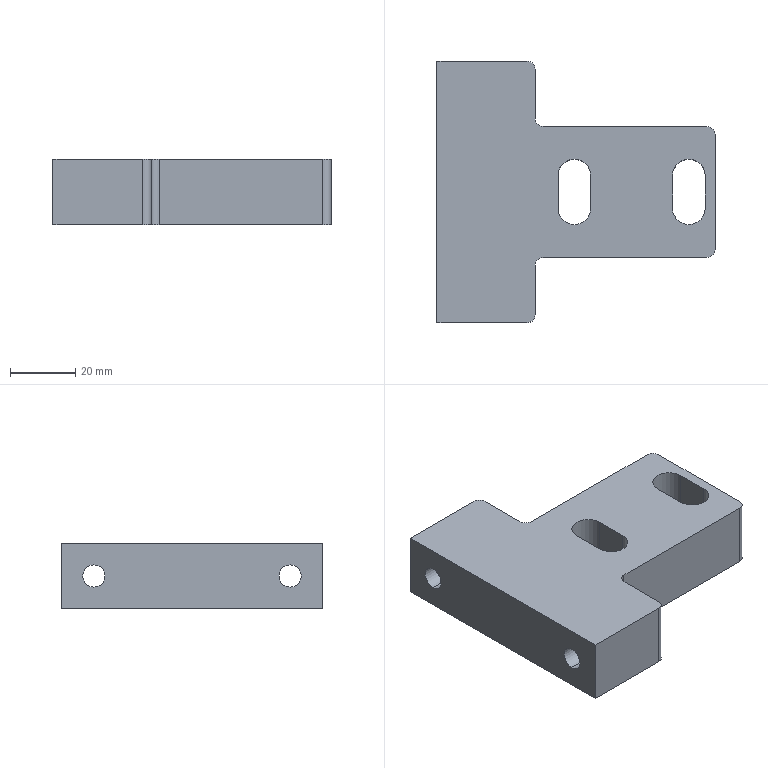Part | 1 solid | 28 faces | box 85 x 80 x 20 mm | volume 82626 mm3 | cylinder 14 | plane 14 | commonest cylinder face diameters 5 x6 6.8 x4 10 x4
STEP:
#1=CARTESIAN_POINT('',(-42.5,30.,13.4));
#2=VERTEX_POINT('',#1);
#3=CARTESIAN_POINT('',(-42.5,30.,6.6));
#4=VERTEX_POINT('',#3);
#5=CARTESIAN_POINT('',(-42.5,30.,10.));
#6=DIRECTION('',(1.,0.,0.));
#7=DIRECTION('',(0.,0.,-1.));
#8=AXIS2_PLACEMENT_3D('',#5,#6,#7);
#9=CIRCLE('',#8,3.4);
#10=EDGE_CURVE('',#2,#4,#9,.T.);
#11=ORIENTED_EDGE('',*,*,#10,.F.);
#12=CARTESIAN_POINT('',(-12.5,30.,13.4));
#13=VERTEX_POINT('',#12);
#14=CARTESIAN_POINT('',(-12.5,30.,13.4));
#15=DIRECTION('',(1.,0.,0.));
#16=VECTOR('',#15,1000.);
#17=LINE('',#14,#16);
#18=EDGE_CURVE('',#2,#13,#17,.T.);
#19=ORIENTED_EDGE('',*,*,#18,.T.);
#20=CARTESIAN_POINT('',(-12.5,30.,6.6));
#21=VERTEX_POINT('',#20);
#22=CARTESIAN_POINT('',(-12.5,30.,10.));
#23=DIRECTION('',(1.,0.,0.));
#24=DIRECTION('',(0.,0.,-1.));
#25=AXIS2_PLACEMENT_3D('',#22,#23,#24);
#26=CIRCLE('',#25,3.4);
#27=EDGE_CURVE('',#13,#21,#26,.T.);
#28=ORIENTED_EDGE('',*,*,#27,.T.);
#29=CARTESIAN_POINT('',(-12.5,30.,6.6));
#30=DIRECTION('',(1.,0.,0.));
#31=VECTOR('',#30,1000.);
#32=LINE('',#29,#31);
#33=EDGE_CURVE('',#4,#21,#32,.T.);
#34=ORIENTED_EDGE('',*,*,#33,.F.);
#35=EDGE_LOOP('',(#11,#19,#28,#34));
#36=FACE_OUTER_BOUND('',#35,.T.);
#37=CARTESIAN_POINT('',(-12.5,30.,10.));
#38=DIRECTION('',(1.,0.,0.));
#39=DIRECTION('',(0.,0.,-1.));
#40=AXIS2_PLACEMENT_3D('',#37,#38,#39);
#41=CYLINDRICAL_SURFACE('',#40,3.4);
#42=ADVANCED_FACE('',(#36),#41,.F.);
#43=CARTESIAN_POINT('',(-42.5,-30.,13.4));
#44=VERTEX_POINT('',#43);
#45=CARTESIAN_POINT('',(-42.5,-30.,6.6));
#46=VERTEX_POINT('',#45);
#47=CARTESIAN_POINT('',(-42.5,-30.,10.));
#48=DIRECTION('',(1.,0.,0.));
#49=DIRECTION('',(0.,0.,-1.));
#50=AXIS2_PLACEMENT_3D('',#47,#48,#49);
#51=CIRCLE('',#50,3.4);
#52=EDGE_CURVE('',#44,#46,#51,.T.);
#53=ORIENTED_EDGE('',*,*,#52,.F.);
#54=CARTESIAN_POINT('',(-12.5,-30.,13.4));
#55=VERTEX_POINT('',#54);
#56=CARTESIAN_POINT('',(-12.5,-30.,13.4));
#57=DIRECTION('',(1.,0.,0.));
#58=VECTOR('',#57,1000.);
#59=LINE('',#56,#58);
#60=EDGE_CURVE('',#44,#55,#59,.T.);
#61=ORIENTED_EDGE('',*,*,#60,.T.);
#62=CARTESIAN_POINT('',(-12.5,-30.,6.6));
#63=VERTEX_POINT('',#62);
#64=CARTESIAN_POINT('',(-12.5,-30.,10.));
#65=DIRECTION('',(1.,0.,0.));
#66=DIRECTION('',(0.,0.,-1.));
#67=AXIS2_PLACEMENT_3D('',#64,#65,#66);
#68=CIRCLE('',#67,3.4);
#69=EDGE_CURVE('',#55,#63,#68,.T.);
#70=ORIENTED_EDGE('',*,*,#69,.T.);
#71=CARTESIAN_POINT('',(-12.5,-30.,6.6));
#72=DIRECTION('',(1.,0.,0.));
#73=VECTOR('',#72,1000.);
#74=LINE('',#71,#73);
#75=EDGE_CURVE('',#46,#63,#74,.T.);
#76=ORIENTED_EDGE('',*,*,#75,.F.);
#77=EDGE_LOOP('',(#53,#61,#70,#76));
#78=FACE_OUTER_BOUND('',#77,.T.);
#79=CARTESIAN_POINT('',(-12.5,-30.,10.));
#80=DIRECTION('',(1.,0.,0.));
#81=DIRECTION('',(0.,0.,-1.));
#82=AXIS2_PLACEMENT_3D('',#79,#80,#81);
#83=CYLINDRICAL_SURFACE('',#82,3.4);
#84=ADVANCED_FACE('',(#78),#83,.F.);
#85=CARTESIAN_POINT('',(-12.5,-22.5,20.));
#86=VERTEX_POINT('',#85);
#87=CARTESIAN_POINT('',(-12.5,-37.5,20.));
#88=VERTEX_POINT('',#87);
#89=CARTESIAN_POINT('',(-12.5,-40.,20.));
#90=DIRECTION('',(0.,-1.,0.));
#91=VECTOR('',#90,1000.);
#92=LINE('',#89,#91);
#93=EDGE_CURVE('',#86,#88,#92,.T.);
#94=ORIENTED_EDGE('',*,*,#93,.T.);
#95=CARTESIAN_POINT('',(-12.5,-37.5,0.));
#96=VERTEX_POINT('',#95);
#97=CARTESIAN_POINT('',(-12.5,-37.5,0.));
#98=DIRECTION('',(0.,0.,-1.));
#99=VECTOR('',#98,1000.);
#100=LINE('',#97,#99);
#101=EDGE_CURVE('',#88,#96,#100,.T.);
#102=ORIENTED_EDGE('',*,*,#101,.T.);
#103=CARTESIAN_POINT('',(-12.5,-22.5,0.));
#104=VERTEX_POINT('',#103);
#105=CARTESIAN_POINT('',(-12.5,-40.,0.));
#106=DIRECTION('',(0.,-1.,0.));
#107=VECTOR('',#106,1000.);
#108=LINE('',#105,#107);
#109=EDGE_CURVE('',#104,#96,#108,.T.);
#110=ORIENTED_EDGE('',*,*,#109,.F.);
#111=CARTESIAN_POINT('',(-12.5,-22.5,20.));
#112=DIRECTION('',(0.,0.,1.));
#113=VECTOR('',#112,1000.);
#114=LINE('',#111,#113);
#115=EDGE_CURVE('',#104,#86,#114,.T.);
#116=ORIENTED_EDGE('',*,*,#115,.T.);
#117=EDGE_LOOP('',(#94,#102,#110,#116));
#118=FACE_OUTER_BOUND('',#117,.T.);
#119=CARTESIAN_POINT('',(-12.5,-30.,10.));
#120=DIRECTION('',(1.,0.,0.));
#121=DIRECTION('',(0.,0.,-1.));
#122=AXIS2_PLACEMENT_3D('',#119,#120,#121);
#123=CIRCLE('',#122,3.4);
#124=EDGE_CURVE('',#63,#55,#123,.T.);
#125=ORIENTED_EDGE('',*,*,#124,.F.);
#126=ORIENTED_EDGE('',*,*,#69,.F.);
#127=EDGE_LOOP('',(#125,#126));
#128=FACE_BOUND('',#127,.T.);
#129=CARTESIAN_POINT('',(-12.5,-40.,0.));
#130=DIRECTION('',(-1.,0.,0.));
#131=DIRECTION('',(0.,0.,1.));
#132=AXIS2_PLACEMENT_3D('',#129,#130,#131);
#133=PLANE('',#132);
#134=ADVANCED_FACE('',(#118,#128),#133,.F.);
#135=CARTESIAN_POINT('',(42.5,-17.5,20.));
#136=VERTEX_POINT('',#135);
#137=CARTESIAN_POINT('',(42.5,17.5,20.));
#138=VERTEX_POINT('',#137);
#139=CARTESIAN_POINT('',(42.5,-40.,20.));
#140=DIRECTION('',(0.,1.,0.));
#141=VECTOR('',#140,1000.);
#142=LINE('',#139,#141);
#143=EDGE_CURVE('',#136,#138,#142,.T.);
#144=ORIENTED_EDGE('',*,*,#143,.F.);
#145=CARTESIAN_POINT('',(42.5,-17.5,0.));
#146=VERTEX_POINT('',#145);
#147=CARTESIAN_POINT('',(42.5,-17.5,20.));
#148=DIRECTION('',(0.,0.,-1.));
#149=VECTOR('',#148,1000.);
#150=LINE('',#147,#149);
#151=EDGE_CURVE('',#136,#146,#150,.T.);
#152=ORIENTED_EDGE('',*,*,#151,.T.);
#153=CARTESIAN_POINT('',(42.5,17.5,0.));
#154=VERTEX_POINT('',#153);
#155=CARTESIAN_POINT('',(42.5,-40.,0.));
#156=DIRECTION('',(0.,1.,0.));
#157=VECTOR('',#156,1000.);
#158=LINE('',#155,#157);
#159=EDGE_CURVE('',#146,#154,#158,.T.);
#160=ORIENTED_EDGE('',*,*,#159,.T.);
#161=CARTESIAN_POINT('',(42.5,17.5,20.));
#162=DIRECTION('',(0.,0.,1.));
#163=VECTOR('',#162,1000.);
#164=LINE('',#161,#163);
#165=EDGE_CURVE('',#154,#138,#164,.T.);
#166=ORIENTED_EDGE('',*,*,#165,.T.);
#167=EDGE_LOOP('',(#144,#152,#160,#166));
#168=FACE_OUTER_BOUND('',#167,.T.);
#169=CARTESIAN_POINT('',(42.5,-40.,20.));
#170=DIRECTION('',(-1.,0.,0.));
#171=DIRECTION('',(0.,0.,1.));
#172=AXIS2_PLACEMENT_3D('',#169,#170,#171);
#173=PLANE('',#172);
#174=ADVANCED_FACE('',(#168),#173,.F.);
#175=CARTESIAN_POINT('',(-15.,40.,20.));
#176=VERTEX_POINT('',#175);
#177=CARTESIAN_POINT('',(-42.5,40.,20.));
#178=VERTEX_POINT('',#177);
#179=CARTESIAN_POINT('',(-42.5,40.,20.));
#180=DIRECTION('',(-1.,0.,0.));
#181=VECTOR('',#180,1000.);
#182=LINE('',#179,#181);
#183=EDGE_CURVE('',#176,#178,#182,.T.);
#184=ORIENTED_EDGE('',*,*,#183,.F.);
#185=CARTESIAN_POINT('',(-15.,40.,0.));
#186=VERTEX_POINT('',#185);
#187=CARTESIAN_POINT('',(-15.,40.,20.));
#188=DIRECTION('',(0.,0.,-1.));
#189=VECTOR('',#188,1000.);
#190=LINE('',#187,#189);
#191=EDGE_CURVE('',#176,#186,#190,.T.);
#192=ORIENTED_EDGE('',*,*,#191,.T.);
#193=CARTESIAN_POINT('',(-42.5,40.,0.));
#194=VERTEX_POINT('',#193);
#195=CARTESIAN_POINT('',(-42.5,40.,0.));
#196=DIRECTION('',(-1.,0.,0.));
#197=VECTOR('',#196,1000.);
#198=LINE('',#195,#197);
#199=EDGE_CURVE('',#186,#194,#198,.T.);
#200=ORIENTED_EDGE('',*,*,#199,.T.);
#201=CARTESIAN_POINT('',(-42.5,40.,20.));
#202=DIRECTION('',(0.,0.,-1.));
#203=VECTOR('',#202,1000.);
#204=LINE('',#201,#203);
#205=EDGE_CURVE('',#178,#194,#204,.T.);
#206=ORIENTED_EDGE('',*,*,#205,.F.);
#207=EDGE_LOOP('',(#184,#192,#200,#206));
#208=FACE_OUTER_BOUND('',#207,.T.);
#209=CARTESIAN_POINT('',(-42.5,40.,20.));
#210=DIRECTION('',(0.,-1.,0.));
#211=DIRECTION('',(0.,0.,-1.));
#212=AXIS2_PLACEMENT_3D('',#209,#210,#211);
#213=PLANE('',#212);
#214=ADVANCED_FACE('',(#208),#213,.F.);
#215=CARTESIAN_POINT('',(-42.5,30.,10.));
#216=DIRECTION('',(1.,0.,0.));
#217=DIRECTION('',(0.,0.,-1.));
#218=AXIS2_PLACEMENT_3D('',#215,#216,#217);
#219=CIRCLE('',#218,3.4);
#220=EDGE_CURVE('',#4,#2,#219,.T.);
#221=ORIENTED_EDGE('',*,*,#220,.T.);
#222=ORIENTED_EDGE('',*,*,#10,.T.);
#223=EDGE_LOOP('',(#221,#222));
#224=FACE_BOUND('',#223,.T.);
#225=CARTESIAN_POINT('',(-42.5,-30.,10.));
#226=DIRECTION('',(1.,0.,0.));
#227=DIRECTION('',(0.,0.,-1.));
#228=AXIS2_PLACEMENT_3D('',#225,#226,#227);
#229=CIRCLE('',#228,3.4);
#230=EDGE_CURVE('',#46,#44,#229,.T.);
#231=ORIENTED_EDGE('',*,*,#230,.T.);
#232=ORIENTED_EDGE('',*,*,#52,.T.);
#233=EDGE_LOOP('',(#231,#232));
#234=FACE_BOUND('',#233,.T.);
#235=CARTESIAN_POINT('',(-42.5,-40.,0.));
#236=VERTEX_POINT('',#235);
#237=CARTESIAN_POINT('',(-42.5,-40.,0.));
#238=DIRECTION('',(0.,-1.,0.));
#239=VECTOR('',#238,1000.);
#240=LINE('',#237,#239);
#241=EDGE_CURVE('',#194,#236,#240,.T.);
#242=ORIENTED_EDGE('',*,*,#241,.T.);
#243=CARTESIAN_POINT('',(-42.5,-40.,20.));
#244=VERTEX_POINT('',#243);
#245=CARTESIAN_POINT('',(-42.5,-40.,20.));
#246=DIRECTION('',(0.,0.,-1.));
#247=VECTOR('',#246,1000.);
#248=LINE('',#245,#247);
#249=EDGE_CURVE('',#244,#236,#248,.T.);
#250=ORIENTED_EDGE('',*,*,#249,.F.);
#251=CARTESIAN_POINT('',(-42.5,-40.,20.));
#252=DIRECTION('',(0.,-1.,0.));
#253=VECTOR('',#252,1000.);
#254=LINE('',#251,#253);
#255=EDGE_CURVE('',#178,#244,#254,.T.);
#256=ORIENTED_EDGE('',*,*,#255,.F.);
#257=ORIENTED_EDGE('',*,*,#205,.T.);
#258=EDGE_LOOP('',(#242,#250,#256,#257));
#259=FACE_OUTER_BOUND('',#258,.T.);
#260=CARTESIAN_POINT('',(-42.5,-40.,20.));
#261=DIRECTION('',(1.,0.,0.));
#262=DIRECTION('',(0.,0.,-1.));
#263=AXIS2_PLACEMENT_3D('',#260,#261,#262);
#264=PLANE('',#263);
#265=ADVANCED_FACE('',(#224,#234,#259),#264,.F.);
#266=CARTESIAN_POINT('',(-15.,-40.,0.));
#267=VERTEX_POINT('',#266);
#268=CARTESIAN_POINT('',(-42.5,-40.,0.));
#269=DIRECTION('',(1.,0.,0.));
#270=VECTOR('',#269,1000.);
#271=LINE('',#268,#270);
#272=EDGE_CURVE('',#236,#267,#271,.T.);
#273=ORIENTED_EDGE('',*,*,#272,.T.);
#274=CARTESIAN_POINT('',(-15.,-40.,20.));
#275=VERTEX_POINT('',#274);
#276=CARTESIAN_POINT('',(-15.,-40.,20.));
#277=DIRECTION('',(0.,0.,1.));
#278=VECTOR('',#277,1000.);
#279=LINE('',#276,#278);
#280=EDGE_CURVE('',#267,#275,#279,.T.);
#281=ORIENTED_EDGE('',*,*,#280,.T.);
#282=CARTESIAN_POINT('',(-42.5,-40.,20.));
#283=DIRECTION('',(1.,0.,0.));
#284=VECTOR('',#283,1000.);
#285=LINE('',#282,#284);
#286=EDGE_CURVE('',#244,#275,#285,.T.);
#287=ORIENTED_EDGE('',*,*,#286,.F.);
#288=ORIENTED_EDGE('',*,*,#249,.T.);
#289=EDGE_LOOP('',(#273,#281,#287,#288));
#290=FACE_OUTER_BOUND('',#289,.T.);
#291=CARTESIAN_POINT('',(-42.5,-40.,20.));
#292=DIRECTION('',(0.,1.,0.));
#293=DIRECTION('',(0.,0.,1.));
#294=AXIS2_PLACEMENT_3D('',#291,#292,#293);
#295=PLANE('',#294);
#296=ADVANCED_FACE('',(#290),#295,.F.);
#297=CARTESIAN_POINT('',(4.5,-5.,20.));
#298=VERTEX_POINT('',#297);
#299=CARTESIAN_POINT('',(4.5,5.,20.));
#300=VERTEX_POINT('',#299);
#301=CARTESIAN_POINT('',(4.5,-5.,20.));
#302=DIRECTION('',(0.,1.,0.));
#303=VECTOR('',#302,1000.);
#304=LINE('',#301,#303);
#305=EDGE_CURVE('',#298,#300,#304,.T.);
#306=ORIENTED_EDGE('',*,*,#305,.F.);
#307=CARTESIAN_POINT('',(-5.5,-5.,20.));
#308=VERTEX_POINT('',#307);
#309=CARTESIAN_POINT('',(-0.5,-5.,20.));
#310=DIRECTION('',(0.,0.,1.));
#311=DIRECTION('',(1.,0.,0.));
#312=AXIS2_PLACEMENT_3D('',#309,#310,#311);
#313=CIRCLE('',#312,5.);
#314=EDGE_CURVE('',#308,#298,#313,.T.);
#315=ORIENTED_EDGE('',*,*,#314,.F.);
#316=CARTESIAN_POINT('',(-5.5,5.,20.));
#317=VERTEX_POINT('',#316);
#318=CARTESIAN_POINT('',(-5.5,-5.,20.));
#319=DIRECTION('',(0.,-1.,0.));
#320=VECTOR('',#319,1000.);
#321=LINE('',#318,#320);
#322=EDGE_CURVE('',#317,#308,#321,.T.);
#323=ORIENTED_EDGE('',*,*,#322,.F.);
#324=CARTESIAN_POINT('',(-0.5,5.,20.));
#325=DIRECTION('',(0.,0.,1.));
#326=DIRECTION('',(1.,0.,0.));
#327=AXIS2_PLACEMENT_3D('',#324,#325,#326);
#328=CIRCLE('',#327,5.);
#329=EDGE_CURVE('',#300,#317,#328,.T.);
#330=ORIENTED_EDGE('',*,*,#329,.F.);
#331=EDGE_LOOP('',(#306,#315,#323,#330));
#332=FACE_BOUND('',#331,.T.);
#333=CARTESIAN_POINT('',(39.5,-5.,20.));
#334=VERTEX_POINT('',#333);
#335=CARTESIAN_POINT('',(39.5,5.,20.));
#336=VERTEX_POINT('',#335);
#337=CARTESIAN_POINT('',(39.5,-5.,20.));
#338=DIRECTION('',(0.,1.,0.));
#339=VECTOR('',#338,1000.);
#340=LINE('',#337,#339);
#341=EDGE_CURVE('',#334,#336,#340,.T.);
#342=ORIENTED_EDGE('',*,*,#341,.F.);
#343=CARTESIAN_POINT('',(29.5,-5.,20.));
#344=VERTEX_POINT('',#343);
#345=CARTESIAN_POINT('',(34.5,-5.,20.));
#346=DIRECTION('',(0.,0.,1.));
#347=DIRECTION('',(1.,0.,0.));
#348=AXIS2_PLACEMENT_3D('',#345,#346,#347);
#349=CIRCLE('',#348,5.);
#350=EDGE_CURVE('',#344,#334,#349,.T.);
#351=ORIENTED_EDGE('',*,*,#350,.F.);
#352=CARTESIAN_POINT('',(29.5,5.,20.));
#353=VERTEX_POINT('',#352);
#354=CARTESIAN_POINT('',(29.5,-5.,20.));
#355=DIRECTION('',(0.,-1.,0.));
#356=VECTOR('',#355,1000.);
#357=LINE('',#354,#356);
#358=EDGE_CURVE('',#353,#344,#357,.T.);
#359=ORIENTED_EDGE('',*,*,#358,.F.);
#360=CARTESIAN_POINT('',(34.5,5.,20.));
#361=DIRECTION('',(0.,0.,1.));
#362=DIRECTION('',(1.,0.,0.));
#363=AXIS2_PLACEMENT_3D('',#360,#361,#362);
#364=CIRCLE('',#363,5.);
#365=EDGE_CURVE('',#336,#353,#364,.T.);
#366=ORIENTED_EDGE('',*,*,#365,.F.);
#367=EDGE_LOOP('',(#342,#351,#359,#366));
#368=FACE_BOUND('',#367,.T.);
#369=CARTESIAN_POINT('',(-12.5,37.5,20.));
#370=VERTEX_POINT('',#369);
#371=CARTESIAN_POINT('',(-12.5,22.5,20.));
#372=VERTEX_POINT('',#371);
#373=CARTESIAN_POINT('',(-12.5,40.,20.));
#374=DIRECTION('',(0.,-1.,0.));
#375=VECTOR('',#374,1000.);
#376=LINE('',#373,#375);
#377=EDGE_CURVE('',#370,#372,#376,.T.);
#378=ORIENTED_EDGE('',*,*,#377,.F.);
#379=CARTESIAN_POINT('',(-15.,37.5,20.));
#380=DIRECTION('',(0.,0.,1.));
#381=DIRECTION('',(-1.,0.,0.));
#382=AXIS2_PLACEMENT_3D('',#379,#380,#381);
#383=CIRCLE('',#382,2.5);
#384=EDGE_CURVE('',#370,#176,#383,.T.);
#385=ORIENTED_EDGE('',*,*,#384,.T.);
#386=ORIENTED_EDGE('',*,*,#183,.T.);
#387=ORIENTED_EDGE('',*,*,#255,.T.);
#388=ORIENTED_EDGE('',*,*,#286,.T.);
#389=CARTESIAN_POINT('',(-15.,-37.5,20.));
#390=DIRECTION('',(0.,0.,1.));
#391=DIRECTION('',(-1.,0.,0.));
#392=AXIS2_PLACEMENT_3D('',#389,#390,#391);
#393=CIRCLE('',#392,2.5);
#394=EDGE_CURVE('',#275,#88,#393,.T.);
#395=ORIENTED_EDGE('',*,*,#394,.T.);
#396=ORIENTED_EDGE('',*,*,#93,.F.);
#397=CARTESIAN_POINT('',(-10.,-20.,20.));
#398=VERTEX_POINT('',#397);
#399=CARTESIAN_POINT('',(-10.,-22.5,20.));
#400=DIRECTION('',(0.,0.,-1.));
#401=DIRECTION('',(-1.,0.,0.));
#402=AXIS2_PLACEMENT_3D('',#399,#400,#401);
#403=CIRCLE('',#402,2.5);
#404=EDGE_CURVE('',#86,#398,#403,.T.);
#405=ORIENTED_EDGE('',*,*,#404,.T.);
#406=CARTESIAN_POINT('',(40.,-20.,20.));
#407=VERTEX_POINT('',#406);
#408=CARTESIAN_POINT('',(42.5,-20.,20.));
#409=DIRECTION('',(-1.,0.,0.));
#410=VECTOR('',#409,1000.);
#411=LINE('',#408,#410);
#412=EDGE_CURVE('',#407,#398,#411,.T.);
#413=ORIENTED_EDGE('',*,*,#412,.F.);
#414=CARTESIAN_POINT('',(40.,-17.5,20.));
#415=DIRECTION('',(0.,0.,1.));
#416=DIRECTION('',(-1.,0.,0.));
#417=AXIS2_PLACEMENT_3D('',#414,#415,#416);
#418=CIRCLE('',#417,2.5);
#419=EDGE_CURVE('',#407,#136,#418,.T.);
#420=ORIENTED_EDGE('',*,*,#419,.T.);
#421=ORIENTED_EDGE('',*,*,#143,.T.);
#422=CARTESIAN_POINT('',(40.,20.,20.));
#423=VERTEX_POINT('',#422);
#424=CARTESIAN_POINT('',(40.,17.5,20.));
#425=DIRECTION('',(0.,0.,1.));
#426=DIRECTION('',(-1.,0.,0.));
#427=AXIS2_PLACEMENT_3D('',#424,#425,#426);
#428=CIRCLE('',#427,2.5);
#429=EDGE_CURVE('',#138,#423,#428,.T.);
#430=ORIENTED_EDGE('',*,*,#429,.T.);
#431=CARTESIAN_POINT('',(-10.,20.,20.));
#432=VERTEX_POINT('',#431);
#433=CARTESIAN_POINT('',(42.5,20.,20.));
#434=DIRECTION('',(1.,0.,0.));
#435=VECTOR('',#434,1000.);
#436=LINE('',#433,#435);
#437=EDGE_CURVE('',#432,#423,#436,.T.);
#438=ORIENTED_EDGE('',*,*,#437,.F.);
#439=CARTESIAN_POINT('',(-10.,22.5,20.));
#440=DIRECTION('',(0.,0.,-1.));
#441=DIRECTION('',(-1.,0.,0.));
#442=AXIS2_PLACEMENT_3D('',#439,#440,#441);
#443=CIRCLE('',#442,2.5);
#444=EDGE_CURVE('',#432,#372,#443,.T.);
#445=ORIENTED_EDGE('',*,*,#444,.T.);
#446=EDGE_LOOP('',(#378,#385,#386,#387,#388,#395,#396,#405,#413,#420,#421,#430,#438,#445));
#447=FACE_OUTER_BOUND('',#446,.T.);
#448=CARTESIAN_POINT('',(0.,0.,20.));
#449=DIRECTION('',(0.,0.,-1.));
#450=DIRECTION('',(-1.,0.,0.));
#451=AXIS2_PLACEMENT_3D('',#448,#449,#450);
#452=PLANE('',#451);
#453=ADVANCED_FACE('',(#332,#368,#447),#452,.F.);
#454=CARTESIAN_POINT('',(-5.5,-5.,0.));
#455=VERTEX_POINT('',#454);
#456=CARTESIAN_POINT('',(4.5,-5.,0.));
#457=VERTEX_POINT('',#456);
#458=CARTESIAN_POINT('',(-0.5,-5.,0.));
#459=DIRECTION('',(0.,0.,1.));
#460=DIRECTION('',(1.,0.,0.));
#461=AXIS2_PLACEMENT_3D('',#458,#459,#460);
#462=CIRCLE('',#461,5.);
#463=EDGE_CURVE('',#455,#457,#462,.T.);
#464=ORIENTED_EDGE('',*,*,#463,.T.);
#465=CARTESIAN_POINT('',(4.5,5.,0.));
#466=VERTEX_POINT('',#465);
#467=CARTESIAN_POINT('',(4.5,-5.,0.));
#468=DIRECTION('',(0.,1.,0.));
#469=VECTOR('',#468,1000.);
#470=LINE('',#467,#469);
#471=EDGE_CURVE('',#457,#466,#470,.T.);
#472=ORIENTED_EDGE('',*,*,#471,.T.);
#473=CARTESIAN_POINT('',(-5.5,5.,0.));
#474=VERTEX_POINT('',#473);
#475=CARTESIAN_POINT('',(-0.5,5.,0.));
#476=DIRECTION('',(0.,0.,1.));
#477=DIRECTION('',(1.,0.,0.));
#478=AXIS2_PLACEMENT_3D('',#475,#476,#477);
#479=CIRCLE('',#478,5.);
#480=EDGE_CURVE('',#466,#474,#479,.T.);
#481=ORIENTED_EDGE('',*,*,#480,.T.);
#482=CARTESIAN_POINT('',(-5.5,-5.,0.));
#483=DIRECTION('',(0.,-1.,0.));
#484=VECTOR('',#483,1000.);
#485=LINE('',#482,#484);
#486=EDGE_CURVE('',#474,#455,#485,.T.);
#487=ORIENTED_EDGE('',*,*,#486,.T.);
#488=EDGE_LOOP('',(#464,#472,#481,#487));
#489=FACE_BOUND('',#488,.T.);
#490=CARTESIAN_POINT('',(29.5,-5.,0.));
#491=VERTEX_POINT('',#490);
#492=CARTESIAN_POINT('',(39.5,-5.,0.));
#493=VERTEX_POINT('',#492);
#494=CARTESIAN_POINT('',(34.5,-5.,0.));
#495=DIRECTION('',(0.,0.,1.));
#496=DIRECTION('',(1.,0.,0.));
#497=AXIS2_PLACEMENT_3D('',#494,#495,#496);
#498=CIRCLE('',#497,5.);
#499=EDGE_CURVE('',#491,#493,#498,.T.);
#500=ORIENTED_EDGE('',*,*,#499,.T.);
#501=CARTESIAN_POINT('',(39.5,5.,0.));
#502=VERTEX_POINT('',#501);
#503=CARTESIAN_POINT('',(39.5,-5.,0.));
#504=DIRECTION('',(0.,1.,0.));
#505=VECTOR('',#504,1000.);
#506=LINE('',#503,#505);
#507=EDGE_CURVE('',#493,#502,#506,.T.);
#508=ORIENTED_EDGE('',*,*,#507,.T.);
#509=CARTESIAN_POINT('',(29.5,5.,0.));
#510=VERTEX_POINT('',#509);
#511=CARTESIAN_POINT('',(34.5,5.,0.));
#512=DIRECTION('',(0.,0.,1.));
#513=DIRECTION('',(1.,0.,0.));
#514=AXIS2_PLACEMENT_3D('',#511,#512,#513);
#515=CIRCLE('',#514,5.);
#516=EDGE_CURVE('',#502,#510,#515,.T.);
#517=ORIENTED_EDGE('',*,*,#516,.T.);
#518=CARTESIAN_POINT('',(29.5,-5.,0.));
#519=DIRECTION('',(0.,-1.,0.));
#520=VECTOR('',#519,1000.);
#521=LINE('',#518,#520);
#522=EDGE_CURVE('',#510,#491,#521,.T.);
#523=ORIENTED_EDGE('',*,*,#522,.T.);
#524=EDGE_LOOP('',(#500,#508,#517,#523));
#525=FACE_BOUND('',#524,.T.);
#526=ORIENTED_EDGE('',*,*,#199,.F.);
#527=CARTESIAN_POINT('',(-12.5,37.5,0.));
#528=VERTEX_POINT('',#527);
#529=CARTESIAN_POINT('',(-15.,37.5,0.));
#530=DIRECTION('',(0.,0.,-1.));
#531=DIRECTION('',(-1.,0.,0.));
#532=AXIS2_PLACEMENT_3D('',#529,#530,#531);
#533=CIRCLE('',#532,2.5);
#534=EDGE_CURVE('',#186,#528,#533,.T.);
#535=ORIENTED_EDGE('',*,*,#534,.T.);
#536=CARTESIAN_POINT('',(-12.5,22.5,0.));
#537=VERTEX_POINT('',#536);
#538=CARTESIAN_POINT('',(-12.5,40.,0.));
#539=DIRECTION('',(0.,-1.,0.));
#540=VECTOR('',#539,1000.);
#541=LINE('',#538,#540);
#542=EDGE_CURVE('',#528,#537,#541,.T.);
#543=ORIENTED_EDGE('',*,*,#542,.T.);
#544=CARTESIAN_POINT('',(-10.,20.,0.));
#545=VERTEX_POINT('',#544);
#546=CARTESIAN_POINT('',(-10.,22.5,0.));
#547=DIRECTION('',(0.,0.,1.));
#548=DIRECTION('',(-1.,0.,0.));
#549=AXIS2_PLACEMENT_3D('',#546,#547,#548);
#550=CIRCLE('',#549,2.5);
#551=EDGE_CURVE('',#537,#545,#550,.T.);
#552=ORIENTED_EDGE('',*,*,#551,.T.);
#553=CARTESIAN_POINT('',(40.,20.,0.));
#554=VERTEX_POINT('',#553);
#555=CARTESIAN_POINT('',(42.5,20.,0.));
#556=DIRECTION('',(1.,0.,0.));
#557=VECTOR('',#556,1000.);
#558=LINE('',#555,#557);
#559=EDGE_CURVE('',#545,#554,#558,.T.);
#560=ORIENTED_EDGE('',*,*,#559,.T.);
#561=CARTESIAN_POINT('',(40.,17.5,0.));
#562=DIRECTION('',(0.,0.,-1.));
#563=DIRECTION('',(-1.,0.,0.));
#564=AXIS2_PLACEMENT_3D('',#561,#562,#563);
#565=CIRCLE('',#564,2.5);
#566=EDGE_CURVE('',#554,#154,#565,.T.);
#567=ORIENTED_EDGE('',*,*,#566,.T.);
#568=ORIENTED_EDGE('',*,*,#159,.F.);
#569=CARTESIAN_POINT('',(40.,-20.,0.));
#570=VERTEX_POINT('',#569);
#571=CARTESIAN_POINT('',(40.,-17.5,0.));
#572=DIRECTION('',(0.,0.,-1.));
#573=DIRECTION('',(-1.,0.,0.));
#574=AXIS2_PLACEMENT_3D('',#571,#572,#573);
#575=CIRCLE('',#574,2.5);
#576=EDGE_CURVE('',#146,#570,#575,.T.);
#577=ORIENTED_EDGE('',*,*,#576,.T.);
#578=CARTESIAN_POINT('',(-10.,-20.,0.));
#579=VERTEX_POINT('',#578);
#580=CARTESIAN_POINT('',(42.5,-20.,0.));
#581=DIRECTION('',(-1.,0.,0.));
#582=VECTOR('',#581,1000.);
#583=LINE('',#580,#582);
#584=EDGE_CURVE('',#570,#579,#583,.T.);
#585=ORIENTED_EDGE('',*,*,#584,.T.);
#586=CARTESIAN_POINT('',(-10.,-22.5,0.));
#587=DIRECTION('',(0.,0.,1.));
#588=DIRECTION('',(-1.,0.,0.));
#589=AXIS2_PLACEMENT_3D('',#586,#587,#588);
#590=CIRCLE('',#589,2.5);
#591=EDGE_CURVE('',#579,#104,#590,.T.);
#592=ORIENTED_EDGE('',*,*,#591,.T.);
#593=ORIENTED_EDGE('',*,*,#109,.T.);
#594=CARTESIAN_POINT('',(-15.,-37.5,0.));
#595=DIRECTION('',(0.,0.,-1.));
#596=DIRECTION('',(-1.,0.,0.));
#597=AXIS2_PLACEMENT_3D('',#594,#595,#596);
#598=CIRCLE('',#597,2.5);
#599=EDGE_CURVE('',#96,#267,#598,.T.);
#600=ORIENTED_EDGE('',*,*,#599,.T.);
#601=ORIENTED_EDGE('',*,*,#272,.F.);
#602=ORIENTED_EDGE('',*,*,#241,.F.);
#603=EDGE_LOOP('',(#526,#535,#543,#552,#560,#567,#568,#577,#585,#592,#593,#600,#601,#602));
#604=FACE_OUTER_BOUND('',#603,.T.);
#605=CARTESIAN_POINT('',(0.,0.,0.));
#606=DIRECTION('',(0.,0.,-1.));
#607=DIRECTION('',(-1.,0.,0.));
#608=AXIS2_PLACEMENT_3D('',#605,#606,#607);
#609=PLANE('',#608);
#610=ADVANCED_FACE('',(#489,#525,#604),#609,.T.);
#611=ORIENTED_EDGE('',*,*,#584,.F.);
#612=CARTESIAN_POINT('',(40.,-20.,0.));
#613=DIRECTION('',(0.,0.,1.));
#614=VECTOR('',#613,1000.);
#615=LINE('',#612,#614);
#616=EDGE_CURVE('',#570,#407,#615,.T.);
#617=ORIENTED_EDGE('',*,*,#616,.T.);
#618=ORIENTED_EDGE('',*,*,#412,.T.);
#619=CARTESIAN_POINT('',(-10.,-20.,0.));
#620=DIRECTION('',(0.,0.,-1.));
#621=VECTOR('',#620,1000.);
#622=LINE('',#619,#621);
#623=EDGE_CURVE('',#398,#579,#622,.T.);
#624=ORIENTED_EDGE('',*,*,#623,.T.);
#625=EDGE_LOOP('',(#611,#617,#618,#624));
#626=FACE_OUTER_BOUND('',#625,.T.);
#627=CARTESIAN_POINT('',(42.5,-20.,0.));
#628=DIRECTION('',(0.,1.,0.));
#629=DIRECTION('',(-1.,0.,0.));
#630=AXIS2_PLACEMENT_3D('',#627,#628,#629);
#631=PLANE('',#630);
#632=ADVANCED_FACE('',(#626),#631,.F.);
#633=ORIENTED_EDGE('',*,*,#559,.F.);
#634=CARTESIAN_POINT('',(-10.,20.,20.));
#635=DIRECTION('',(0.,0.,1.));
#636=VECTOR('',#635,1000.);
#637=LINE('',#634,#636);
#638=EDGE_CURVE('',#545,#432,#637,.T.);
#639=ORIENTED_EDGE('',*,*,#638,.T.);
#640=ORIENTED_EDGE('',*,*,#437,.T.);
#641=CARTESIAN_POINT('',(40.,20.,0.));
#642=DIRECTION('',(0.,0.,-1.));
#643=VECTOR('',#642,1000.);
#644=LINE('',#641,#643);
#645=EDGE_CURVE('',#423,#554,#644,.T.);
#646=ORIENTED_EDGE('',*,*,#645,.T.);
#647=EDGE_LOOP('',(#633,#639,#640,#646));
#648=FACE_OUTER_BOUND('',#647,.T.);
#649=CARTESIAN_POINT('',(42.5,20.,0.));
#650=DIRECTION('',(0.,-1.,0.));
#651=DIRECTION('',(1.,0.,0.));
#652=AXIS2_PLACEMENT_3D('',#649,#650,#651);
#653=PLANE('',#652);
#654=ADVANCED_FACE('',(#648),#653,.F.);
#655=CARTESIAN_POINT('',(-12.5,30.,10.));
#656=DIRECTION('',(1.,0.,0.));
#657=DIRECTION('',(0.,0.,-1.));
#658=AXIS2_PLACEMENT_3D('',#655,#656,#657);
#659=CIRCLE('',#658,3.4);
#660=EDGE_CURVE('',#21,#13,#659,.T.);
#661=ORIENTED_EDGE('',*,*,#660,.F.);
#662=ORIENTED_EDGE('',*,*,#27,.F.);
#663=EDGE_LOOP('',(#661,#662));
#664=FACE_BOUND('',#663,.T.);
#665=ORIENTED_EDGE('',*,*,#377,.T.);
#666=CARTESIAN_POINT('',(-12.5,22.5,0.));
#667=DIRECTION('',(0.,0.,-1.));
#668=VECTOR('',#667,1000.);
#669=LINE('',#666,#668);
#670=EDGE_CURVE('',#372,#537,#669,.T.);
#671=ORIENTED_EDGE('',*,*,#670,.T.);
#672=ORIENTED_EDGE('',*,*,#542,.F.);
#673=CARTESIAN_POINT('',(-12.5,37.5,0.));
#674=DIRECTION('',(0.,0.,1.));
#675=VECTOR('',#674,1000.);
#676=LINE('',#673,#675);
#677=EDGE_CURVE('',#528,#370,#676,.T.);
#678=ORIENTED_EDGE('',*,*,#677,.T.);
#679=EDGE_LOOP('',(#665,#671,#672,#678));
#680=FACE_OUTER_BOUND('',#679,.T.);
#681=CARTESIAN_POINT('',(-12.5,40.,0.));
#682=DIRECTION('',(-1.,0.,0.));
#683=DIRECTION('',(0.,-1.,0.));
#684=AXIS2_PLACEMENT_3D('',#681,#682,#683);
#685=PLANE('',#684);
#686=ADVANCED_FACE('',(#664,#680),#685,.F.);
#687=ORIENTED_EDGE('',*,*,#350,.T.);
#688=CARTESIAN_POINT('',(39.5,-5.,0.));
#689=DIRECTION('',(0.,0.,1.));
#690=VECTOR('',#689,1000.);
#691=LINE('',#688,#690);
#692=EDGE_CURVE('',#493,#334,#691,.T.);
#693=ORIENTED_EDGE('',*,*,#692,.F.);
#694=ORIENTED_EDGE('',*,*,#499,.F.);
#695=CARTESIAN_POINT('',(29.5,-5.,0.));
#696=DIRECTION('',(0.,0.,1.));
#697=VECTOR('',#696,1000.);
#698=LINE('',#695,#697);
#699=EDGE_CURVE('',#491,#344,#698,.T.);
#700=ORIENTED_EDGE('',*,*,#699,.T.);
#701=EDGE_LOOP('',(#687,#693,#694,#700));
#702=FACE_OUTER_BOUND('',#701,.T.);
#703=CARTESIAN_POINT('',(34.5,-5.,0.));
#704=DIRECTION('',(0.,0.,1.));
#705=DIRECTION('',(1.,0.,0.));
#706=AXIS2_PLACEMENT_3D('',#703,#704,#705);
#707=CYLINDRICAL_SURFACE('',#706,5.);
#708=ADVANCED_FACE('',(#702),#707,.F.);
#709=ORIENTED_EDGE('',*,*,#358,.T.);
#710=ORIENTED_EDGE('',*,*,#699,.F.);
#711=ORIENTED_EDGE('',*,*,#522,.F.);
#712=CARTESIAN_POINT('',(29.5,5.,0.));
#713=DIRECTION('',(0.,0.,1.));
#714=VECTOR('',#713,1000.);
#715=LINE('',#712,#714);
#716=EDGE_CURVE('',#510,#353,#715,.T.);
#717=ORIENTED_EDGE('',*,*,#716,.T.);
#718=EDGE_LOOP('',(#709,#710,#711,#717));
#719=FACE_OUTER_BOUND('',#718,.T.);
#720=CARTESIAN_POINT('',(29.5,-5.,0.));
#721=DIRECTION('',(-1.,0.,0.));
#722=DIRECTION('',(0.,0.,1.));
#723=AXIS2_PLACEMENT_3D('',#720,#721,#722);
#724=PLANE('',#723);
#725=ADVANCED_FACE('',(#719),#724,.F.);
#726=ORIENTED_EDGE('',*,*,#365,.T.);
#727=ORIENTED_EDGE('',*,*,#716,.F.);
#728=ORIENTED_EDGE('',*,*,#516,.F.);
#729=CARTESIAN_POINT('',(39.5,5.,0.));
#730=DIRECTION('',(0.,0.,1.));
#731=VECTOR('',#730,1000.);
#732=LINE('',#729,#731);
#733=EDGE_CURVE('',#502,#336,#732,.T.);
#734=ORIENTED_EDGE('',*,*,#733,.T.);
#735=EDGE_LOOP('',(#726,#727,#728,#734));
#736=FACE_OUTER_BOUND('',#735,.T.);
#737=CARTESIAN_POINT('',(34.5,5.,0.));
#738=DIRECTION('',(0.,0.,1.));
#739=DIRECTION('',(1.,0.,0.));
#740=AXIS2_PLACEMENT_3D('',#737,#738,#739);
#741=CYLINDRICAL_SURFACE('',#740,5.);
#742=ADVANCED_FACE('',(#736),#741,.F.);
#743=ORIENTED_EDGE('',*,*,#341,.T.);
#744=ORIENTED_EDGE('',*,*,#733,.F.);
#745=ORIENTED_EDGE('',*,*,#507,.F.);
#746=ORIENTED_EDGE('',*,*,#692,.T.);
#747=EDGE_LOOP('',(#743,#744,#745,#746));
#748=FACE_OUTER_BOUND('',#747,.T.);
#749=CARTESIAN_POINT('',(39.5,-5.,0.));
#750=DIRECTION('',(1.,0.,0.));
#751=DIRECTION('',(0.,0.,-1.));
#752=AXIS2_PLACEMENT_3D('',#749,#750,#751);
#753=PLANE('',#752);
#754=ADVANCED_FACE('',(#748),#753,.F.);
#755=ORIENTED_EDGE('',*,*,#314,.T.);
#756=CARTESIAN_POINT('',(4.5,-5.,0.));
#757=DIRECTION('',(0.,0.,1.));
#758=VECTOR('',#757,1000.);
#759=LINE('',#756,#758);
#760=EDGE_CURVE('',#457,#298,#759,.T.);
#761=ORIENTED_EDGE('',*,*,#760,.F.);
#762=ORIENTED_EDGE('',*,*,#463,.F.);
#763=CARTESIAN_POINT('',(-5.5,-5.,0.));
#764=DIRECTION('',(0.,0.,1.));
#765=VECTOR('',#764,1000.);
#766=LINE('',#763,#765);
#767=EDGE_CURVE('',#455,#308,#766,.T.);
#768=ORIENTED_EDGE('',*,*,#767,.T.);
#769=EDGE_LOOP('',(#755,#761,#762,#768));
#770=FACE_OUTER_BOUND('',#769,.T.);
#771=CARTESIAN_POINT('',(-0.5,-5.,0.));
#772=DIRECTION('',(0.,0.,1.));
#773=DIRECTION('',(1.,0.,0.));
#774=AXIS2_PLACEMENT_3D('',#771,#772,#773);
#775=CYLINDRICAL_SURFACE('',#774,5.);
#776=ADVANCED_FACE('',(#770),#775,.F.);
#777=ORIENTED_EDGE('',*,*,#322,.T.);
#778=ORIENTED_EDGE('',*,*,#767,.F.);
#779=ORIENTED_EDGE('',*,*,#486,.F.);
#780=CARTESIAN_POINT('',(-5.5,5.,0.));
#781=DIRECTION('',(0.,0.,1.));
#782=VECTOR('',#781,1000.);
#783=LINE('',#780,#782);
#784=EDGE_CURVE('',#474,#317,#783,.T.);
#785=ORIENTED_EDGE('',*,*,#784,.T.);
#786=EDGE_LOOP('',(#777,#778,#779,#785));
#787=FACE_OUTER_BOUND('',#786,.T.);
#788=CARTESIAN_POINT('',(-5.5,-5.,0.));
#789=DIRECTION('',(-1.,0.,0.));
#790=DIRECTION('',(0.,0.,1.));
#791=AXIS2_PLACEMENT_3D('',#788,#789,#790);
#792=PLANE('',#791);
#793=ADVANCED_FACE('',(#787),#792,.F.);
#794=ORIENTED_EDGE('',*,*,#329,.T.);
#795=ORIENTED_EDGE('',*,*,#784,.F.);
#796=ORIENTED_EDGE('',*,*,#480,.F.);
#797=CARTESIAN_POINT('',(4.5,5.,0.));
#798=DIRECTION('',(0.,0.,1.));
#799=VECTOR('',#798,1000.);
#800=LINE('',#797,#799);
#801=EDGE_CURVE('',#466,#300,#800,.T.);
#802=ORIENTED_EDGE('',*,*,#801,.T.);
#803=EDGE_LOOP('',(#794,#795,#796,#802));
#804=FACE_OUTER_BOUND('',#803,.T.);
#805=CARTESIAN_POINT('',(-0.5,5.,0.));
#806=DIRECTION('',(0.,0.,1.));
#807=DIRECTION('',(1.,0.,0.));
#808=AXIS2_PLACEMENT_3D('',#805,#806,#807);
#809=CYLINDRICAL_SURFACE('',#808,5.);
#810=ADVANCED_FACE('',(#804),#809,.F.);
#811=ORIENTED_EDGE('',*,*,#305,.T.);
#812=ORIENTED_EDGE('',*,*,#801,.F.);
#813=ORIENTED_EDGE('',*,*,#471,.F.);
#814=ORIENTED_EDGE('',*,*,#760,.T.);
#815=EDGE_LOOP('',(#811,#812,#813,#814));
#816=FACE_OUTER_BOUND('',#815,.T.);
#817=CARTESIAN_POINT('',(4.5,-5.,0.));
#818=DIRECTION('',(1.,0.,0.));
#819=DIRECTION('',(0.,0.,-1.));
#820=AXIS2_PLACEMENT_3D('',#817,#818,#819);
#821=PLANE('',#820);
#822=ADVANCED_FACE('',(#816),#821,.F.);
#823=ORIENTED_EDGE('',*,*,#60,.F.);
#824=ORIENTED_EDGE('',*,*,#230,.F.);
#825=ORIENTED_EDGE('',*,*,#75,.T.);
#826=ORIENTED_EDGE('',*,*,#124,.T.);
#827=EDGE_LOOP('',(#823,#824,#825,#826));
#828=FACE_OUTER_BOUND('',#827,.T.);
#829=CARTESIAN_POINT('',(-12.5,-30.,10.));
#830=DIRECTION('',(1.,0.,0.));
#831=DIRECTION('',(0.,0.,-1.));
#832=AXIS2_PLACEMENT_3D('',#829,#830,#831);
#833=CYLINDRICAL_SURFACE('',#832,3.4);
#834=ADVANCED_FACE('',(#828),#833,.F.);
#835=ORIENTED_EDGE('',*,*,#18,.F.);
#836=ORIENTED_EDGE('',*,*,#220,.F.);
#837=ORIENTED_EDGE('',*,*,#33,.T.);
#838=ORIENTED_EDGE('',*,*,#660,.T.);
#839=EDGE_LOOP('',(#835,#836,#837,#838));
#840=FACE_OUTER_BOUND('',#839,.T.);
#841=CARTESIAN_POINT('',(-12.5,30.,10.));
#842=DIRECTION('',(1.,0.,0.));
#843=DIRECTION('',(0.,0.,-1.));
#844=AXIS2_PLACEMENT_3D('',#841,#842,#843);
#845=CYLINDRICAL_SURFACE('',#844,3.4);
#846=ADVANCED_FACE('',(#840),#845,.F.);
#847=ORIENTED_EDGE('',*,*,#551,.F.);
#848=ORIENTED_EDGE('',*,*,#670,.F.);
#849=ORIENTED_EDGE('',*,*,#444,.F.);
#850=ORIENTED_EDGE('',*,*,#638,.F.);
#851=EDGE_LOOP('',(#847,#848,#849,#850));
#852=FACE_OUTER_BOUND('',#851,.T.);
#853=CARTESIAN_POINT('',(-10.,22.5,0.));
#854=DIRECTION('',(0.,0.,-1.));
#855=DIRECTION('',(-1.,0.,0.));
#856=AXIS2_PLACEMENT_3D('',#853,#854,#855);
#857=CYLINDRICAL_SURFACE('',#856,2.5);
#858=ADVANCED_FACE('',(#852),#857,.F.);
#859=ORIENTED_EDGE('',*,*,#534,.F.);
#860=ORIENTED_EDGE('',*,*,#191,.F.);
#861=ORIENTED_EDGE('',*,*,#384,.F.);
#862=ORIENTED_EDGE('',*,*,#677,.F.);
#863=EDGE_LOOP('',(#859,#860,#861,#862));
#864=FACE_OUTER_BOUND('',#863,.T.);
#865=CARTESIAN_POINT('',(-15.,37.5,0.));
#866=DIRECTION('',(0.,0.,1.));
#867=DIRECTION('',(1.,0.,0.));
#868=AXIS2_PLACEMENT_3D('',#865,#866,#867);
#869=CYLINDRICAL_SURFACE('',#868,2.5);
#870=ADVANCED_FACE('',(#864),#869,.T.);
#871=ORIENTED_EDGE('',*,*,#599,.F.);
#872=ORIENTED_EDGE('',*,*,#101,.F.);
#873=ORIENTED_EDGE('',*,*,#394,.F.);
#874=ORIENTED_EDGE('',*,*,#280,.F.);
#875=EDGE_LOOP('',(#871,#872,#873,#874));
#876=FACE_OUTER_BOUND('',#875,.T.);
#877=CARTESIAN_POINT('',(-15.,-37.5,20.));
#878=DIRECTION('',(0.,0.,1.));
#879=DIRECTION('',(1.,0.,0.));
#880=AXIS2_PLACEMENT_3D('',#877,#878,#879);
#881=CYLINDRICAL_SURFACE('',#880,2.5);
#882=ADVANCED_FACE('',(#876),#881,.T.);
#883=ORIENTED_EDGE('',*,*,#576,.F.);
#884=ORIENTED_EDGE('',*,*,#151,.F.);
#885=ORIENTED_EDGE('',*,*,#419,.F.);
#886=ORIENTED_EDGE('',*,*,#616,.F.);
#887=EDGE_LOOP('',(#883,#884,#885,#886));
#888=FACE_OUTER_BOUND('',#887,.T.);
#889=CARTESIAN_POINT('',(40.,-17.5,0.));
#890=DIRECTION('',(0.,0.,1.));
#891=DIRECTION('',(1.,0.,0.));
#892=AXIS2_PLACEMENT_3D('',#889,#890,#891);
#893=CYLINDRICAL_SURFACE('',#892,2.5);
#894=ADVANCED_FACE('',(#888),#893,.T.);
#895=ORIENTED_EDGE('',*,*,#566,.F.);
#896=ORIENTED_EDGE('',*,*,#645,.F.);
#897=ORIENTED_EDGE('',*,*,#429,.F.);
#898=ORIENTED_EDGE('',*,*,#165,.F.);
#899=EDGE_LOOP('',(#895,#896,#897,#898));
#900=FACE_OUTER_BOUND('',#899,.T.);
#901=CARTESIAN_POINT('',(40.,17.5,20.));
#902=DIRECTION('',(0.,0.,1.));
#903=DIRECTION('',(1.,0.,0.));
#904=AXIS2_PLACEMENT_3D('',#901,#902,#903);
#905=CYLINDRICAL_SURFACE('',#904,2.5);
#906=ADVANCED_FACE('',(#900),#905,.T.);
#907=ORIENTED_EDGE('',*,*,#591,.F.);
#908=ORIENTED_EDGE('',*,*,#623,.F.);
#909=ORIENTED_EDGE('',*,*,#404,.F.);
#910=ORIENTED_EDGE('',*,*,#115,.F.);
#911=EDGE_LOOP('',(#907,#908,#909,#910));
#912=FACE_OUTER_BOUND('',#911,.T.);
#913=CARTESIAN_POINT('',(-10.,-22.5,0.));
#914=DIRECTION('',(0.,0.,-1.));
#915=DIRECTION('',(-1.,0.,0.));
#916=AXIS2_PLACEMENT_3D('',#913,#914,#915);
#917=CYLINDRICAL_SURFACE('',#916,2.5);
#918=ADVANCED_FACE('',(#912),#917,.F.);
#919=CLOSED_SHELL('',(#42,#84,#134,#174,#214,#265,#296,#453,#610,#632,#654,#686,#708,#725,#742,#754,#776,#793,#810,#822,#834,#846,#858,#870,#882,#894,#906,#918));
#920=MANIFOLD_SOLID_BREP('',#919);
#921=CARTESIAN_POINT('',(0.,0.,0.));
#922=DIRECTION('',(0.,0.,1.));
#923=DIRECTION('',(1.,0.,0.));
#924=AXIS2_PLACEMENT_3D('',#921,#922,#923);
#925=(LENGTH_UNIT()NAMED_UNIT(*)SI_UNIT(.MILLI.,.METRE.));
#926=UNCERTAINTY_MEASURE_WITH_UNIT(LENGTH_MEASURE(0.00001),#925,'','');
#927=(NAMED_UNIT(*)PLANE_ANGLE_UNIT()SI_UNIT($,.RADIAN.));
#928=(NAMED_UNIT(*)SI_UNIT($,.STERADIAN.)SOLID_ANGLE_UNIT());
#929=(GEOMETRIC_REPRESENTATION_CONTEXT(3)GLOBAL_UNCERTAINTY_ASSIGNED_CONTEXT((#926))GLOBAL_UNIT_ASSIGNED_CONTEXT((#925,#927,#928))REPRESENTATION_CONTEXT('',''));
#930=ADVANCED_BREP_SHAPE_REPRESENTATION('',(#920,#924),#929);